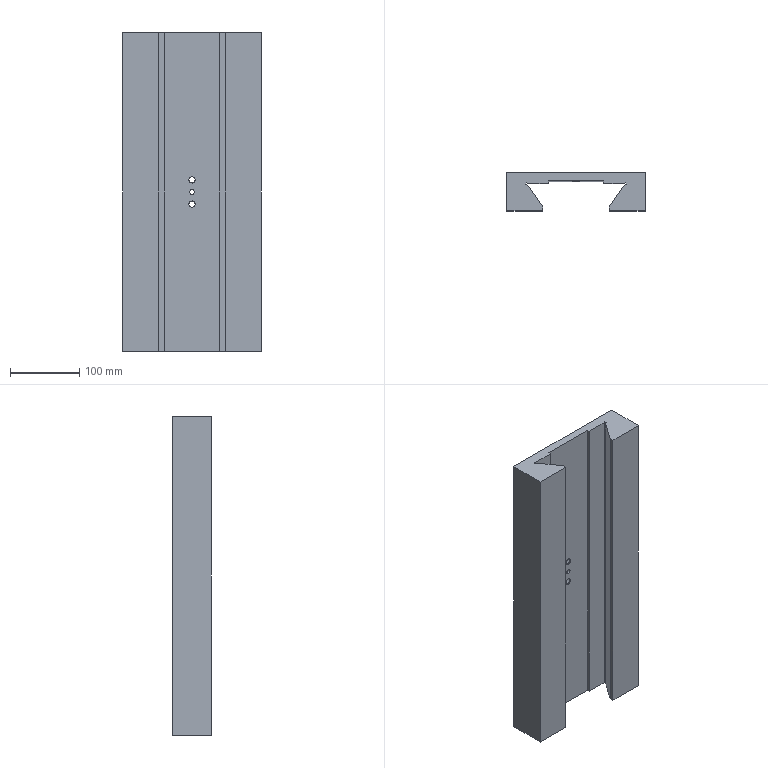Part | SolidWorks | features HoleWzd 2, Extrusion 1 | 1 solid | 82 faces | box 200 x 55 x 460 mm | volume 2781667 mm3 | cylinder 34 | cone 24 | plane 24 | commonest cylinder face diameters 6.8 x26 9 x4 18 x4